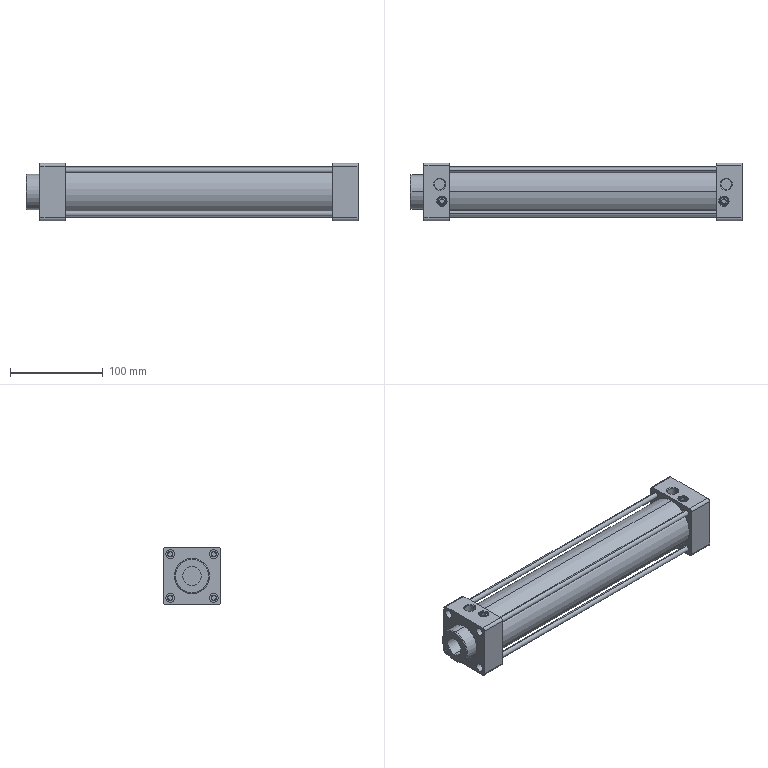Part | SolidWorks | features BaseBody 1 | 1 solid | 147 faces | box 358 x 62 x 62 mm | volume 348569 mm3 | cylinder 76 | plane 41 | cone 28 | torus 2 | commonest cylinder face diameters 4.917 x16 6 x16 9.5 x16 5 x4 9.1 x4 10.1 x4